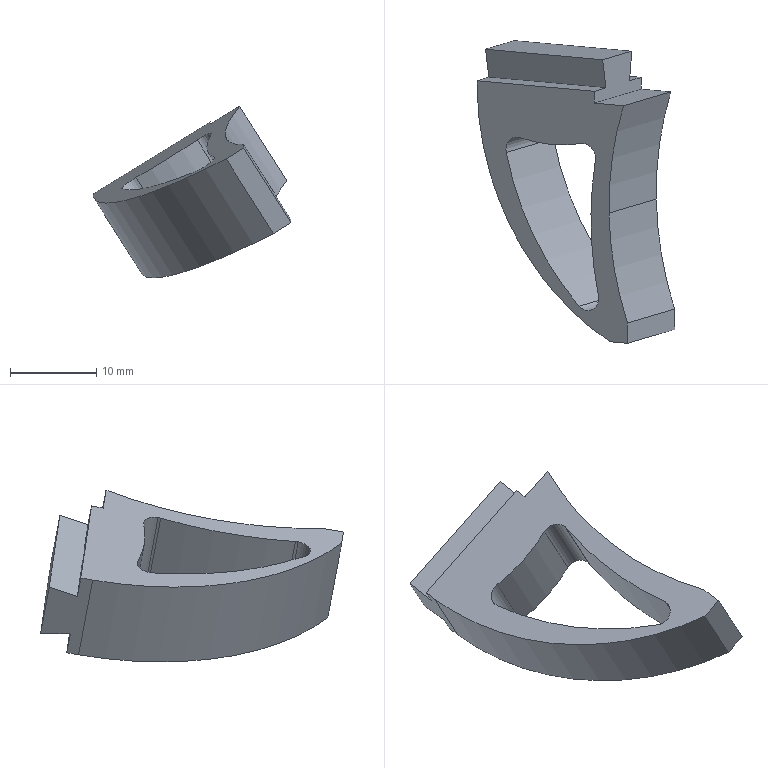Part | SolidWorks | features SplitBody 1 | 1 solid | 23 faces | box 22.985 x 35.159 x 19.952 mm | volume 2822 mm3 | plane 12 | cylinder 11 | commonest cylinder face diameters 3.2 x5 75.2 x2 40 x1 63.431 x1 67.2 x1 80 x1
STEP:
#1=CARTESIAN_POINT('',(526.695,281.026,-373.992));
#2=VERTEX_POINT('',#1);
#3=CARTESIAN_POINT('',(526.675,280.725,-374.062));
#4=VERTEX_POINT('',#3);
#5=CARTESIAN_POINT('',(525.336,281.15,-374.827));
#6=DIRECTION('',(0.5274,0.157,-0.835));
#7=DIRECTION('',(0.8494,-0.07732,0.522));
#8=AXIS2_PLACEMENT_3D('',#5,#6,#7);
#9=CIRCLE('',#8,1.6);
#10=EDGE_CURVE('',#2,#4,#9,.T.);
#11=ORIENTED_EDGE('',*,*,#10,.F.);
#12=CARTESIAN_POINT('',(532.181,282.659,-382.676));
#13=VERTEX_POINT('',#12);
#14=CARTESIAN_POINT('',(526.695,281.026,-373.992));
#15=DIRECTION('',(0.5274,0.157,-0.835));
#16=VECTOR('',#15,1000.);
#17=LINE('',#14,#16);
#18=EDGE_CURVE('',#2,#13,#17,.T.);
#19=ORIENTED_EDGE('',*,*,#18,.T.);
#20=CARTESIAN_POINT('',(532.161,282.358,-382.745));
#21=VERTEX_POINT('',#20);
#22=CARTESIAN_POINT('',(530.822,282.783,-383.511));
#23=DIRECTION('',(0.5274,0.157,-0.835));
#24=DIRECTION('',(0.8494,-0.07732,0.522));
#25=AXIS2_PLACEMENT_3D('',#22,#23,#24);
#26=CIRCLE('',#25,1.6);
#27=EDGE_CURVE('',#13,#21,#26,.T.);
#28=ORIENTED_EDGE('',*,*,#27,.T.);
#29=CARTESIAN_POINT('',(526.675,280.725,-374.062));
#30=DIRECTION('',(0.5274,0.157,-0.835));
#31=VECTOR('',#30,1000.);
#32=LINE('',#29,#31);
#33=EDGE_CURVE('',#4,#21,#32,.T.);
#34=ORIENTED_EDGE('',*,*,#33,.F.);
#35=EDGE_LOOP('',(#11,#19,#28,#34));
#36=FACE_OUTER_BOUND('',#35,.T.);
#37=CARTESIAN_POINT('',(525.336,281.15,-374.827));
#38=DIRECTION('',(0.5274,0.157,-0.835));
#39=DIRECTION('',(0.8494,-0.07732,0.522));
#40=AXIS2_PLACEMENT_3D('',#37,#38,#39);
#41=CYLINDRICAL_SURFACE('',#40,1.6);
#42=ADVANCED_FACE('',(#36),#41,.F.);
#43=CARTESIAN_POINT('',(524.781,263.843,-378.433));
#44=VERTEX_POINT('',#43);
#45=CARTESIAN_POINT('',(527.063,264.768,-376.818));
#46=VERTEX_POINT('',#45);
#47=CARTESIAN_POINT('',(525.703,264.892,-377.653));
#48=DIRECTION('',(-0.5274,-0.157,0.835));
#49=DIRECTION('',(0.8494,-0.07732,0.522));
#50=AXIS2_PLACEMENT_3D('',#47,#48,#49);
#51=CIRCLE('',#50,1.6);
#52=EDGE_CURVE('',#44,#46,#51,.T.);
#53=ORIENTED_EDGE('',*,*,#52,.T.);
#54=CARTESIAN_POINT('',(532.548,266.401,-385.501));
#55=VERTEX_POINT('',#54);
#56=CARTESIAN_POINT('',(527.063,264.768,-376.818));
#57=DIRECTION('',(0.5274,0.157,-0.835));
#58=VECTOR('',#57,1000.);
#59=LINE('',#56,#58);
#60=EDGE_CURVE('',#46,#55,#59,.T.);
#61=ORIENTED_EDGE('',*,*,#60,.T.);
#62=CARTESIAN_POINT('',(530.266,265.476,-387.117));
#63=VERTEX_POINT('',#62);
#64=CARTESIAN_POINT('',(531.189,266.525,-386.337));
#65=DIRECTION('',(-0.5274,-0.157,0.835));
#66=DIRECTION('',(0.8494,-0.07732,0.522));
#67=AXIS2_PLACEMENT_3D('',#64,#65,#66);
#68=CIRCLE('',#67,1.6);
#69=EDGE_CURVE('',#63,#55,#68,.T.);
#70=ORIENTED_EDGE('',*,*,#69,.F.);
#71=CARTESIAN_POINT('',(524.781,263.843,-378.433));
#72=DIRECTION('',(0.5274,0.157,-0.835));
#73=VECTOR('',#72,1000.);
#74=LINE('',#71,#73);
#75=EDGE_CURVE('',#44,#63,#74,.T.);
#76=ORIENTED_EDGE('',*,*,#75,.F.);
#77=EDGE_LOOP('',(#53,#61,#70,#76));
#78=FACE_OUTER_BOUND('',#77,.T.);
#79=CARTESIAN_POINT('',(525.703,264.892,-377.653));
#80=DIRECTION('',(0.5274,0.157,-0.835));
#81=DIRECTION('',(0.8494,-0.07732,0.522));
#82=AXIS2_PLACEMENT_3D('',#79,#80,#81);
#83=CYLINDRICAL_SURFACE('',#82,1.6);
#84=ADVANCED_FACE('',(#78),#83,.F.);
#85=CARTESIAN_POINT('',(533.75,276.287,-382.883));
#86=VERTEX_POINT('',#85);
#87=CARTESIAN_POINT('',(535.88,263.511,-383.94));
#88=VERTEX_POINT('',#87);
#89=CARTESIAN_POINT('',(565.688,273.38,-363.255));
#90=DIRECTION('',(-0.5274,-0.157,0.835));
#91=DIRECTION('',(0.8494,-0.07732,0.522));
#92=AXIS2_PLACEMENT_3D('',#89,#90,#91);
#93=CIRCLE('',#92,37.6);
#94=EDGE_CURVE('',#86,#88,#93,.T.);
#95=ORIENTED_EDGE('',*,*,#94,.F.);
#96=CARTESIAN_POINT('',(528.264,274.654,-374.199));
#97=VERTEX_POINT('',#96);
#98=CARTESIAN_POINT('',(533.75,276.287,-382.883));
#99=DIRECTION('',(-0.5274,-0.157,0.835));
#100=VECTOR('',#99,1000.);
#101=LINE('',#98,#100);
#102=EDGE_CURVE('',#86,#97,#101,.T.);
#103=ORIENTED_EDGE('',*,*,#102,.T.);
#104=CARTESIAN_POINT('',(530.395,261.878,-375.256));
#105=VERTEX_POINT('',#104);
#106=CARTESIAN_POINT('',(560.203,271.747,-354.571));
#107=DIRECTION('',(-0.5274,-0.157,0.835));
#108=DIRECTION('',(0.8494,-0.07732,0.522));
#109=AXIS2_PLACEMENT_3D('',#106,#107,#108);
#110=CIRCLE('',#109,37.6);
#111=EDGE_CURVE('',#97,#105,#110,.T.);
#112=ORIENTED_EDGE('',*,*,#111,.T.);
#113=CARTESIAN_POINT('',(535.88,263.511,-383.94));
#114=DIRECTION('',(-0.5274,-0.157,0.835));
#115=VECTOR('',#114,1000.);
#116=LINE('',#113,#115);
#117=EDGE_CURVE('',#88,#105,#116,.T.);
#118=ORIENTED_EDGE('',*,*,#117,.F.);
#119=EDGE_LOOP('',(#95,#103,#112,#118));
#120=FACE_OUTER_BOUND('',#119,.T.);
#121=CARTESIAN_POINT('',(565.688,273.38,-363.255));
#122=DIRECTION('',(-0.5274,-0.157,0.835));
#123=DIRECTION('',(-0.8494,0.07732,-0.522));
#124=AXIS2_PLACEMENT_3D('',#121,#122,#123);
#125=CYLINDRICAL_SURFACE('',#124,37.6);
#126=ADVANCED_FACE('',(#120),#125,.F.);
#127=CARTESIAN_POINT('',(512.961,288.629,-381.238));
#128=VERTEX_POINT('',#127);
#129=CARTESIAN_POINT('',(528.398,259.701,-376.927));
#130=VERTEX_POINT('',#129);
#131=CARTESIAN_POINT('',(539.892,286.573,-364.613));
#132=DIRECTION('',(-0.5274,-0.157,0.835));
#133=DIRECTION('',(0.8494,-0.07732,0.522));
#134=AXIS2_PLACEMENT_3D('',#131,#132,#133);
#135=CIRCLE('',#134,31.716);
#136=EDGE_CURVE('',#128,#130,#135,.T.);
#137=ORIENTED_EDGE('',*,*,#136,.F.);
#138=CARTESIAN_POINT('',(518.446,290.262,-389.922));
#139=VERTEX_POINT('',#138);
#140=CARTESIAN_POINT('',(518.446,290.262,-389.922));
#141=DIRECTION('',(-0.5274,-0.157,0.835));
#142=VECTOR('',#141,1000.);
#143=LINE('',#140,#142);
#144=EDGE_CURVE('',#139,#128,#143,.T.);
#145=ORIENTED_EDGE('',*,*,#144,.F.);
#146=CARTESIAN_POINT('',(533.883,261.334,-385.611));
#147=VERTEX_POINT('',#146);
#148=CARTESIAN_POINT('',(545.377,288.206,-373.297));
#149=DIRECTION('',(-0.5274,-0.157,0.835));
#150=DIRECTION('',(0.8494,-0.07732,0.522));
#151=AXIS2_PLACEMENT_3D('',#148,#149,#150);
#152=CIRCLE('',#151,31.716);
#153=EDGE_CURVE('',#139,#147,#152,.T.);
#154=ORIENTED_EDGE('',*,*,#153,.T.);
#155=CARTESIAN_POINT('',(533.883,261.334,-385.611));
#156=DIRECTION('',(-0.5274,-0.157,0.835));
#157=VECTOR('',#156,1000.);
#158=LINE('',#155,#157);
#159=EDGE_CURVE('',#147,#130,#158,.T.);
#160=ORIENTED_EDGE('',*,*,#159,.T.);
#161=EDGE_LOOP('',(#137,#145,#154,#160));
#162=FACE_OUTER_BOUND('',#161,.T.);
#163=CARTESIAN_POINT('',(545.377,288.206,-373.297));
#164=DIRECTION('',(-0.5274,-0.157,0.835));
#165=DIRECTION('',(-0.8494,0.07732,-0.522));
#166=AXIS2_PLACEMENT_3D('',#163,#164,#165);
#167=CYLINDRICAL_SURFACE('',#166,31.716);
#168=ADVANCED_FACE('',(#162),#167,.T.);
#169=CARTESIAN_POINT('',(517.051,291.23,-387.508));
#170=VERTEX_POINT('',#169);
#171=CARTESIAN_POINT('',(517.308,294.674,-387.416));
#172=VERTEX_POINT('',#171);
#173=CARTESIAN_POINT('',(517.051,291.23,-387.508));
#174=DIRECTION('',(0.07444,0.9969,0.02652));
#175=VECTOR('',#174,1000.);
#176=LINE('',#173,#175);
#177=EDGE_CURVE('',#170,#172,#176,.T.);
#178=ORIENTED_EDGE('',*,*,#177,.F.);
#179=CARTESIAN_POINT('',(518.422,291.638,-389.679));
#180=VERTEX_POINT('',#179);
#181=CARTESIAN_POINT('',(518.422,291.638,-389.679));
#182=DIRECTION('',(-0.5274,-0.157,0.835));
#183=VECTOR('',#182,1000.);
#184=LINE('',#181,#183);
#185=EDGE_CURVE('',#180,#170,#184,.T.);
#186=ORIENTED_EDGE('',*,*,#185,.F.);
#187=CARTESIAN_POINT('',(518.363,294.988,-389.086));
#188=DIRECTION('',(0.01741,-0.9846,-0.1742));
#189=VECTOR('',#188,1000.);
#190=LINE('',#187,#189);
#191=EDGE_CURVE('',#180,#139,#190,.T.);
#192=ORIENTED_EDGE('',*,*,#191,.T.);
#193=ORIENTED_EDGE('',*,*,#144,.T.);
#194=CARTESIAN_POINT('',(512.937,290.005,-380.995));
#195=VERTEX_POINT('',#194);
#196=CARTESIAN_POINT('',(512.877,293.355,-380.402));
#197=DIRECTION('',(0.01741,-0.9846,-0.1742));
#198=VECTOR('',#197,1000.);
#199=LINE('',#196,#198);
#200=EDGE_CURVE('',#195,#128,#199,.T.);
#201=ORIENTED_EDGE('',*,*,#200,.F.);
#202=CARTESIAN_POINT('',(514.308,290.413,-383.166));
#203=VERTEX_POINT('',#202);
#204=CARTESIAN_POINT('',(512.937,290.005,-380.995));
#205=DIRECTION('',(-0.5274,-0.157,0.835));
#206=VECTOR('',#205,1000.);
#207=LINE('',#204,#206);
#208=EDGE_CURVE('',#203,#195,#207,.T.);
#209=ORIENTED_EDGE('',*,*,#208,.F.);
#210=CARTESIAN_POINT('',(513.932,293.669,-382.072));
#211=VERTEX_POINT('',#210);
#212=CARTESIAN_POINT('',(514.308,290.413,-383.166));
#213=DIRECTION('',(0.1087,-0.9423,-0.3165));
#214=VECTOR('',#213,1000.);
#215=LINE('',#212,#214);
#216=EDGE_CURVE('',#211,#203,#215,.T.);
#217=ORIENTED_EDGE('',*,*,#216,.F.);
#218=CARTESIAN_POINT('',(518.363,294.988,-389.086));
#219=DIRECTION('',(-0.5274,-0.157,0.835));
#220=VECTOR('',#219,1000.);
#221=LINE('',#218,#220);
#222=EDGE_CURVE('',#172,#211,#221,.T.);
#223=ORIENTED_EDGE('',*,*,#222,.F.);
#224=EDGE_LOOP('',(#178,#186,#192,#193,#201,#209,#217,#223));
#225=FACE_OUTER_BOUND('',#224,.T.);
#226=CARTESIAN_POINT('',(518.363,294.988,-389.086));
#227=DIRECTION('',(-0.8494,0.07732,-0.522));
#228=DIRECTION('',(0.5274,0.157,-0.835));
#229=AXIS2_PLACEMENT_3D('',#226,#227,#228);
#230=PLANE('',#229);
#231=ADVANCED_FACE('',(#225),#230,.T.);
#232=CARTESIAN_POINT('',(530.899,293.437,-379.064));
#233=VERTEX_POINT('',#232);
#234=CARTESIAN_POINT('',(527.523,292.432,-373.72));
#235=VERTEX_POINT('',#234);
#236=CARTESIAN_POINT('',(531.953,293.751,-380.734));
#237=DIRECTION('',(-0.5274,-0.157,0.835));
#238=VECTOR('',#237,1000.);
#239=LINE('',#236,#238);
#240=EDGE_CURVE('',#233,#235,#239,.T.);
#241=ORIENTED_EDGE('',*,*,#240,.F.);
#242=CARTESIAN_POINT('',(534.296,293.128,-376.976));
#243=DIRECTION('',(-0.8494,0.07732,-0.522));
#244=VECTOR('',#243,1000.);
#245=LINE('',#242,#244);
#246=EDGE_CURVE('',#233,#172,#245,.T.);
#247=ORIENTED_EDGE('',*,*,#246,.T.);
#248=ORIENTED_EDGE('',*,*,#222,.T.);
#249=CARTESIAN_POINT('',(530.921,292.123,-371.632));
#250=DIRECTION('',(-0.8494,0.07732,-0.522));
#251=VECTOR('',#250,1000.);
#252=LINE('',#249,#251);
#253=EDGE_CURVE('',#235,#211,#252,.T.);
#254=ORIENTED_EDGE('',*,*,#253,.F.);
#255=EDGE_LOOP('',(#241,#247,#248,#254));
#256=FACE_OUTER_BOUND('',#255,.T.);
#257=CARTESIAN_POINT('',(518.363,294.988,-389.086));
#258=DIRECTION('',(0.01741,-0.9846,-0.1742));
#259=DIRECTION('',(-0.8494,0.07732,-0.522));
#260=AXIS2_PLACEMENT_3D('',#257,#258,#259);
#261=PLANE('',#260);
#262=ADVANCED_FACE('',(#256),#261,.F.);
#263=CARTESIAN_POINT('',(532.013,290.401,-381.326));
#264=VERTEX_POINT('',#263);
#265=CARTESIAN_POINT('',(530.641,289.992,-379.155));
#266=VERTEX_POINT('',#265);
#267=CARTESIAN_POINT('',(532.013,290.401,-381.326));
#268=DIRECTION('',(-0.5274,-0.157,0.835));
#269=VECTOR('',#268,1000.);
#270=LINE('',#267,#269);
#271=EDGE_CURVE('',#264,#266,#270,.T.);
#272=ORIENTED_EDGE('',*,*,#271,.T.);
#273=CARTESIAN_POINT('',(530.924,293.783,-379.054));
#274=DIRECTION('',(0.07444,0.9969,0.02652));
#275=VECTOR('',#274,1000.);
#276=LINE('',#273,#275);
#277=EDGE_CURVE('',#266,#233,#276,.T.);
#278=ORIENTED_EDGE('',*,*,#277,.T.);
#279=ORIENTED_EDGE('',*,*,#240,.T.);
#280=CARTESIAN_POINT('',(527.899,289.176,-374.814));
#281=VERTEX_POINT('',#280);
#282=CARTESIAN_POINT('',(527.682,291.057,-374.182));
#283=DIRECTION('',(0.1087,-0.9423,-0.3165));
#284=VECTOR('',#283,1000.);
#285=LINE('',#282,#284);
#286=EDGE_CURVE('',#235,#281,#285,.T.);
#287=ORIENTED_EDGE('',*,*,#286,.T.);
#288=CARTESIAN_POINT('',(526.527,288.768,-372.643));
#289=VERTEX_POINT('',#288);
#290=CARTESIAN_POINT('',(532.013,290.401,-381.326));
#291=DIRECTION('',(-0.5274,-0.157,0.835));
#292=VECTOR('',#291,1000.);
#293=LINE('',#290,#292);
#294=EDGE_CURVE('',#281,#289,#293,.T.);
#295=ORIENTED_EDGE('',*,*,#294,.T.);
#296=CARTESIAN_POINT('',(526.552,287.392,-372.886));
#297=VERTEX_POINT('',#296);
#298=CARTESIAN_POINT('',(526.468,292.118,-372.05));
#299=DIRECTION('',(0.01741,-0.9846,-0.1742));
#300=VECTOR('',#299,1000.);
#301=LINE('',#298,#300);
#302=EDGE_CURVE('',#289,#297,#301,.T.);
#303=ORIENTED_EDGE('',*,*,#302,.T.);
#304=CARTESIAN_POINT('',(532.037,289.025,-381.57));
#305=VERTEX_POINT('',#304);
#306=CARTESIAN_POINT('',(532.037,289.025,-381.57));
#307=DIRECTION('',(-0.5274,-0.157,0.835));
#308=VECTOR('',#307,1000.);
#309=LINE('',#306,#308);
#310=EDGE_CURVE('',#305,#297,#309,.T.);
#311=ORIENTED_EDGE('',*,*,#310,.F.);
#312=CARTESIAN_POINT('',(531.953,293.751,-380.734));
#313=DIRECTION('',(0.01741,-0.9846,-0.1742));
#314=VECTOR('',#313,1000.);
#315=LINE('',#312,#314);
#316=EDGE_CURVE('',#264,#305,#315,.T.);
#317=ORIENTED_EDGE('',*,*,#316,.F.);
#318=EDGE_LOOP('',(#272,#278,#279,#287,#295,#303,#311,#317));
#319=FACE_OUTER_BOUND('',#318,.T.);
#320=CARTESIAN_POINT('',(531.953,293.751,-380.734));
#321=DIRECTION('',(-0.8494,0.07732,-0.522));
#322=DIRECTION('',(0.5274,0.157,-0.835));
#323=AXIS2_PLACEMENT_3D('',#320,#321,#322);
#324=PLANE('',#323);
#325=ADVANCED_FACE('',(#319),#324,.F.);
#326=CARTESIAN_POINT('',(529.949,287.083,-370.798));
#327=VERTEX_POINT('',#326);
#328=CARTESIAN_POINT('',(512.961,288.629,-381.238));
#329=DIRECTION('',(0.8494,-0.07732,0.522));
#330=VECTOR('',#329,1000.);
#331=LINE('',#328,#330);
#332=EDGE_CURVE('',#297,#327,#331,.T.);
#333=ORIENTED_EDGE('',*,*,#332,.T.);
#334=CARTESIAN_POINT('',(535.435,288.716,-379.481));
#335=VERTEX_POINT('',#334);
#336=CARTESIAN_POINT('',(535.435,288.716,-379.481));
#337=DIRECTION('',(-0.5274,-0.157,0.835));
#338=VECTOR('',#337,1000.);
#339=LINE('',#336,#338);
#340=EDGE_CURVE('',#335,#327,#339,.T.);
#341=ORIENTED_EDGE('',*,*,#340,.F.);
#342=CARTESIAN_POINT('',(518.446,290.262,-389.922));
#343=DIRECTION('',(0.8494,-0.07732,0.522));
#344=VECTOR('',#343,1000.);
#345=LINE('',#342,#344);
#346=EDGE_CURVE('',#305,#335,#345,.T.);
#347=ORIENTED_EDGE('',*,*,#346,.F.);
#348=ORIENTED_EDGE('',*,*,#310,.T.);
#349=EDGE_LOOP('',(#333,#341,#347,#348));
#350=FACE_OUTER_BOUND('',#349,.T.);
#351=CARTESIAN_POINT('',(518.446,290.262,-389.922));
#352=DIRECTION('',(0.01741,-0.9846,-0.1742));
#353=DIRECTION('',(-0.8494,0.07732,-0.522));
#354=AXIS2_PLACEMENT_3D('',#351,#352,#353);
#355=PLANE('',#354);
#356=ADVANCED_FACE('',(#350),#355,.F.);
#357=ORIENTED_EDGE('',*,*,#102,.F.);
#358=CARTESIAN_POINT('',(565.688,273.38,-363.255));
#359=DIRECTION('',(-0.5274,-0.157,0.835));
#360=DIRECTION('',(0.8494,-0.07732,0.522));
#361=AXIS2_PLACEMENT_3D('',#358,#359,#360);
#362=CIRCLE('',#361,37.6);
#363=EDGE_CURVE('',#335,#86,#362,.T.);
#364=ORIENTED_EDGE('',*,*,#363,.F.);
#365=ORIENTED_EDGE('',*,*,#340,.T.);
#366=CARTESIAN_POINT('',(560.203,271.747,-354.571));
#367=DIRECTION('',(-0.5274,-0.157,0.835));
#368=DIRECTION('',(0.8494,-0.07732,0.522));
#369=AXIS2_PLACEMENT_3D('',#366,#367,#368);
#370=CIRCLE('',#369,37.6);
#371=EDGE_CURVE('',#327,#97,#370,.T.);
#372=ORIENTED_EDGE('',*,*,#371,.T.);
#373=EDGE_LOOP('',(#357,#364,#365,#372));
#374=FACE_OUTER_BOUND('',#373,.T.);
#375=CARTESIAN_POINT('',(565.688,273.38,-363.255));
#376=DIRECTION('',(-0.5274,-0.157,0.835));
#377=DIRECTION('',(-0.8494,0.07732,-0.522));
#378=AXIS2_PLACEMENT_3D('',#375,#376,#377);
#379=CYLINDRICAL_SURFACE('',#378,37.6);
#380=ADVANCED_FACE('',(#374),#379,.F.);
#381=CARTESIAN_POINT('',(530.437,259.515,-375.674));
#382=VERTEX_POINT('',#381);
#383=CARTESIAN_POINT('',(529.866,291.809,-369.962));
#384=DIRECTION('',(0.01741,-0.9846,-0.1742));
#385=VECTOR('',#384,1000.);
#386=LINE('',#383,#385);
#387=EDGE_CURVE('',#105,#382,#386,.T.);
#388=ORIENTED_EDGE('',*,*,#387,.T.);
#389=CARTESIAN_POINT('',(535.922,261.148,-384.358));
#390=VERTEX_POINT('',#389);
#391=CARTESIAN_POINT('',(535.922,261.148,-384.358));
#392=DIRECTION('',(-0.5274,-0.157,0.835));
#393=VECTOR('',#392,1000.);
#394=LINE('',#391,#393);
#395=EDGE_CURVE('',#390,#382,#394,.T.);
#396=ORIENTED_EDGE('',*,*,#395,.F.);
#397=CARTESIAN_POINT('',(535.351,293.442,-378.645));
#398=DIRECTION('',(0.01741,-0.9846,-0.1742));
#399=VECTOR('',#398,1000.);
#400=LINE('',#397,#399);
#401=EDGE_CURVE('',#88,#390,#400,.T.);
#402=ORIENTED_EDGE('',*,*,#401,.F.);
#403=ORIENTED_EDGE('',*,*,#117,.T.);
#404=EDGE_LOOP('',(#388,#396,#402,#403));
#405=FACE_OUTER_BOUND('',#404,.T.);
#406=CARTESIAN_POINT('',(535.351,293.442,-378.645));
#407=DIRECTION('',(-0.8494,0.07732,-0.522));
#408=DIRECTION('',(0.5274,0.157,-0.835));
#409=AXIS2_PLACEMENT_3D('',#406,#407,#408);
#410=PLANE('',#409);
#411=ADVANCED_FACE('',(#405),#410,.F.);
#412=CARTESIAN_POINT('',(513.448,261.061,-386.115));
#413=DIRECTION('',(-0.8494,0.07732,-0.522));
#414=VECTOR('',#413,1000.);
#415=LINE('',#412,#414);
#416=EDGE_CURVE('',#382,#130,#415,.T.);
#417=ORIENTED_EDGE('',*,*,#416,.T.);
#418=ORIENTED_EDGE('',*,*,#159,.F.);
#419=CARTESIAN_POINT('',(518.934,262.694,-394.798));
#420=DIRECTION('',(-0.8494,0.07732,-0.522));
#421=VECTOR('',#420,1000.);
#422=LINE('',#419,#421);
#423=EDGE_CURVE('',#390,#147,#422,.T.);
#424=ORIENTED_EDGE('',*,*,#423,.F.);
#425=ORIENTED_EDGE('',*,*,#395,.T.);
#426=EDGE_LOOP('',(#417,#418,#424,#425));
#427=FACE_OUTER_BOUND('',#426,.T.);
#428=CARTESIAN_POINT('',(518.934,262.694,-394.798));
#429=DIRECTION('',(-0.01741,0.9846,0.1742));
#430=DIRECTION('',(0.8494,-0.07732,0.522));
#431=AXIS2_PLACEMENT_3D('',#428,#429,#430);
#432=PLANE('',#431);
#433=ADVANCED_FACE('',(#427),#432,.F.);
#434=CARTESIAN_POINT('',(521.816,283.318,-389.1));
#435=VERTEX_POINT('',#434);
#436=CARTESIAN_POINT('',(549.64,287.505,-370.736));
#437=DIRECTION('',(-0.5274,-0.157,0.835));
#438=DIRECTION('',(0.8494,-0.07732,0.522));
#439=AXIS2_PLACEMENT_3D('',#436,#437,#438);
#440=CIRCLE('',#439,33.6);
#441=EDGE_CURVE('',#435,#63,#440,.T.);
#442=ORIENTED_EDGE('',*,*,#441,.T.);
#443=ORIENTED_EDGE('',*,*,#69,.T.);
#444=CARTESIAN_POINT('',(532.514,266.725,-385.462));
#445=VERTEX_POINT('',#444);
#446=CARTESIAN_POINT('',(531.189,266.525,-386.337));
#447=DIRECTION('',(-0.5274,-0.157,0.835));
#448=DIRECTION('',(0.8494,-0.07732,0.522));
#449=AXIS2_PLACEMENT_3D('',#446,#447,#448);
#450=CIRCLE('',#449,1.6);
#451=EDGE_CURVE('',#55,#445,#450,.T.);
#452=ORIENTED_EDGE('',*,*,#451,.T.);
#453=CARTESIAN_POINT('',(565.634,271.73,-363.599));
#454=DIRECTION('',(0.5274,0.157,-0.835));
#455=DIRECTION('',(0.8494,-0.07732,0.522));
#456=AXIS2_PLACEMENT_3D('',#453,#454,#455);
#457=CIRCLE('',#456,40.);
#458=EDGE_CURVE('',#445,#21,#457,.T.);
#459=ORIENTED_EDGE('',*,*,#458,.T.);
#460=ORIENTED_EDGE('',*,*,#27,.F.);
#461=CARTESIAN_POINT('',(530.515,284.35,-383.41));
#462=VERTEX_POINT('',#461);
#463=CARTESIAN_POINT('',(530.822,282.783,-383.511));
#464=DIRECTION('',(0.5274,0.157,-0.835));
#465=DIRECTION('',(0.8494,-0.07732,0.522));
#466=AXIS2_PLACEMENT_3D('',#463,#464,#465);
#467=CIRCLE('',#466,1.6);
#468=EDGE_CURVE('',#462,#13,#467,.T.);
#469=ORIENTED_EDGE('',*,*,#468,.F.);
#470=CARTESIAN_POINT('',(523.403,285.031,-387.775));
#471=VERTEX_POINT('',#470);
#472=CARTESIAN_POINT('',(526.685,303.939,-382.146));
#473=DIRECTION('',(-0.5274,-0.157,0.835));
#474=DIRECTION('',(0.8494,-0.07732,0.522));
#475=AXIS2_PLACEMENT_3D('',#472,#473,#474);
#476=CIRCLE('',#475,20.);
#477=EDGE_CURVE('',#471,#462,#476,.T.);
#478=ORIENTED_EDGE('',*,*,#477,.F.);
#479=CARTESIAN_POINT('',(523.14,283.518,-388.225));
#480=DIRECTION('',(-0.5274,-0.157,0.835));
#481=DIRECTION('',(0.8494,-0.07732,0.522));
#482=AXIS2_PLACEMENT_3D('',#479,#480,#481);
#483=CIRCLE('',#482,1.6);
#484=EDGE_CURVE('',#471,#435,#483,.T.);
#485=ORIENTED_EDGE('',*,*,#484,.T.);
#486=EDGE_LOOP('',(#442,#443,#452,#459,#460,#469,#478,#485));
#487=FACE_BOUND('',#486,.T.);
#488=CARTESIAN_POINT('',(518.422,291.638,-389.679));
#489=DIRECTION('',(-0.8494,0.07732,-0.522));
#490=VECTOR('',#489,1000.);
#491=LINE('',#488,#490);
#492=EDGE_CURVE('',#264,#180,#491,.T.);
#493=ORIENTED_EDGE('',*,*,#492,.F.);
#494=ORIENTED_EDGE('',*,*,#316,.T.);
#495=ORIENTED_EDGE('',*,*,#346,.T.);
#496=ORIENTED_EDGE('',*,*,#363,.T.);
#497=ORIENTED_EDGE('',*,*,#94,.T.);
#498=ORIENTED_EDGE('',*,*,#401,.T.);
#499=ORIENTED_EDGE('',*,*,#423,.T.);
#500=ORIENTED_EDGE('',*,*,#153,.F.);
#501=ORIENTED_EDGE('',*,*,#191,.F.);
#502=EDGE_LOOP('',(#493,#494,#495,#496,#497,#498,#499,#500,#501));
#503=FACE_OUTER_BOUND('',#502,.T.);
#504=CARTESIAN_POINT('',(518.363,294.988,-389.086));
#505=DIRECTION('',(0.5274,0.157,-0.835));
#506=DIRECTION('',(0.8494,-0.07732,0.522));
#507=AXIS2_PLACEMENT_3D('',#504,#505,#506);
#508=PLANE('',#507);
#509=ADVANCED_FACE('',(#487,#503),#508,.T.);
#510=ORIENTED_EDGE('',*,*,#52,.F.);
#511=CARTESIAN_POINT('',(516.33,281.685,-380.416));
#512=VERTEX_POINT('',#511);
#513=CARTESIAN_POINT('',(544.155,285.872,-362.052));
#514=DIRECTION('',(-0.5274,-0.157,0.835));
#515=DIRECTION('',(0.8494,-0.07732,0.522));
#516=AXIS2_PLACEMENT_3D('',#513,#514,#515);
#517=CIRCLE('',#516,33.6);
#518=EDGE_CURVE('',#512,#44,#517,.T.);
#519=ORIENTED_EDGE('',*,*,#518,.F.);
#520=CARTESIAN_POINT('',(517.918,283.398,-379.091));
#521=VERTEX_POINT('',#520);
#522=CARTESIAN_POINT('',(517.655,281.885,-379.541));
#523=DIRECTION('',(-0.5274,-0.157,0.835));
#524=DIRECTION('',(0.8494,-0.07732,0.522));
#525=AXIS2_PLACEMENT_3D('',#522,#523,#524);
#526=CIRCLE('',#525,1.6);
#527=EDGE_CURVE('',#521,#512,#526,.T.);
#528=ORIENTED_EDGE('',*,*,#527,.F.);
#529=CARTESIAN_POINT('',(525.03,282.717,-374.726));
#530=VERTEX_POINT('',#529);
#531=CARTESIAN_POINT('',(521.2,302.306,-373.462));
#532=DIRECTION('',(-0.5274,-0.157,0.835));
#533=DIRECTION('',(0.8494,-0.07732,0.522));
#534=AXIS2_PLACEMENT_3D('',#531,#532,#533);
#535=CIRCLE('',#534,20.);
#536=EDGE_CURVE('',#521,#530,#535,.T.);
#537=ORIENTED_EDGE('',*,*,#536,.T.);
#538=CARTESIAN_POINT('',(525.336,281.15,-374.827));
#539=DIRECTION('',(0.5274,0.157,-0.835));
#540=DIRECTION('',(0.8494,-0.07732,0.522));
#541=AXIS2_PLACEMENT_3D('',#538,#539,#540);
#542=CIRCLE('',#541,1.6);
#543=EDGE_CURVE('',#530,#2,#542,.T.);
#544=ORIENTED_EDGE('',*,*,#543,.T.);
#545=ORIENTED_EDGE('',*,*,#10,.T.);
#546=CARTESIAN_POINT('',(527.028,265.092,-376.779));
#547=VERTEX_POINT('',#546);
#548=CARTESIAN_POINT('',(560.149,270.097,-354.916));
#549=DIRECTION('',(0.5274,0.157,-0.835));
#550=DIRECTION('',(0.8494,-0.07732,0.522));
#551=AXIS2_PLACEMENT_3D('',#548,#549,#550);
#552=CIRCLE('',#551,40.);
#553=EDGE_CURVE('',#547,#4,#552,.T.);
#554=ORIENTED_EDGE('',*,*,#553,.F.);
#555=CARTESIAN_POINT('',(525.703,264.892,-377.653));
#556=DIRECTION('',(-0.5274,-0.157,0.835));
#557=DIRECTION('',(0.8494,-0.07732,0.522));
#558=AXIS2_PLACEMENT_3D('',#555,#556,#557);
#559=CIRCLE('',#558,1.6);
#560=EDGE_CURVE('',#46,#547,#559,.T.);
#561=ORIENTED_EDGE('',*,*,#560,.F.);
#562=EDGE_LOOP('',(#510,#519,#528,#537,#544,#545,#554,#561));
#563=FACE_BOUND('',#562,.T.);
#564=ORIENTED_EDGE('',*,*,#302,.F.);
#565=CARTESIAN_POINT('',(512.937,290.005,-380.995));
#566=DIRECTION('',(-0.8494,0.07732,-0.522));
#567=VECTOR('',#566,1000.);
#568=LINE('',#565,#567);
#569=EDGE_CURVE('',#289,#195,#568,.T.);
#570=ORIENTED_EDGE('',*,*,#569,.T.);
#571=ORIENTED_EDGE('',*,*,#200,.T.);
#572=ORIENTED_EDGE('',*,*,#136,.T.);
#573=ORIENTED_EDGE('',*,*,#416,.F.);
#574=ORIENTED_EDGE('',*,*,#387,.F.);
#575=ORIENTED_EDGE('',*,*,#111,.F.);
#576=ORIENTED_EDGE('',*,*,#371,.F.);
#577=ORIENTED_EDGE('',*,*,#332,.F.);
#578=EDGE_LOOP('',(#564,#570,#571,#572,#573,#574,#575,#576,#577));
#579=FACE_OUTER_BOUND('',#578,.T.);
#580=CARTESIAN_POINT('',(512.877,293.355,-380.402));
#581=DIRECTION('',(0.5274,0.157,-0.835));
#582=DIRECTION('',(0.8494,-0.07732,0.522));
#583=AXIS2_PLACEMENT_3D('',#580,#581,#582);
#584=PLANE('',#583);
#585=ADVANCED_FACE('',(#563,#579),#584,.F.);
#586=ORIENTED_EDGE('',*,*,#253,.T.);
#587=ORIENTED_EDGE('',*,*,#216,.T.);
#588=CARTESIAN_POINT('',(531.296,288.867,-372.725));
#589=DIRECTION('',(-0.8494,0.07732,-0.522));
#590=VECTOR('',#589,1000.);
#591=LINE('',#588,#590);
#592=EDGE_CURVE('',#281,#203,#591,.T.);
#593=ORIENTED_EDGE('',*,*,#592,.F.);
#594=ORIENTED_EDGE('',*,*,#286,.F.);
#595=EDGE_LOOP('',(#586,#587,#593,#594));
#596=FACE_OUTER_BOUND('',#595,.T.);
#597=CARTESIAN_POINT('',(531.296,288.867,-372.725));
#598=DIRECTION('',(0.5164,0.3256,-0.792));
#599=DIRECTION('',(0.1087,-0.9423,-0.3165));
#600=AXIS2_PLACEMENT_3D('',#597,#598,#599);
#601=PLANE('',#600);
#602=ADVANCED_FACE('',(#596),#601,.F.);
#603=ORIENTED_EDGE('',*,*,#592,.T.);
#604=ORIENTED_EDGE('',*,*,#208,.T.);
#605=ORIENTED_EDGE('',*,*,#569,.F.);
#606=ORIENTED_EDGE('',*,*,#294,.F.);
#607=EDGE_LOOP('',(#603,#604,#605,#606));
#608=FACE_OUTER_BOUND('',#607,.T.);
#609=CARTESIAN_POINT('',(529.925,288.458,-370.555));
#610=DIRECTION('',(0.01741,-0.9846,-0.1742));
#611=DIRECTION('',(-0.5274,-0.157,0.835));
#612=AXIS2_PLACEMENT_3D('',#609,#610,#611);
#613=PLANE('',#612);
#614=ADVANCED_FACE('',(#608),#613,.F.);
#615=CARTESIAN_POINT('',(534.039,289.683,-377.067));
#616=DIRECTION('',(-0.8494,0.07732,-0.522));
#617=VECTOR('',#616,1000.);
#618=LINE('',#615,#617);
#619=EDGE_CURVE('',#266,#170,#618,.T.);
#620=ORIENTED_EDGE('',*,*,#619,.T.);
#621=ORIENTED_EDGE('',*,*,#177,.T.);
#622=ORIENTED_EDGE('',*,*,#246,.F.);
#623=ORIENTED_EDGE('',*,*,#277,.F.);
#624=EDGE_LOOP('',(#620,#621,#622,#623));
#625=FACE_OUTER_BOUND('',#624,.T.);
#626=CARTESIAN_POINT('',(534.039,289.683,-377.067));
#627=DIRECTION('',(-0.5224,0.01633,0.8525));
#628=DIRECTION('',(0.07444,0.9969,0.02652));
#629=AXIS2_PLACEMENT_3D('',#626,#627,#628);
#630=PLANE('',#629);
#631=ADVANCED_FACE('',(#625),#630,.F.);
#632=ORIENTED_EDGE('',*,*,#492,.T.);
#633=ORIENTED_EDGE('',*,*,#185,.T.);
#634=ORIENTED_EDGE('',*,*,#619,.F.);
#635=ORIENTED_EDGE('',*,*,#271,.F.);
#636=EDGE_LOOP('',(#632,#633,#634,#635));
#637=FACE_OUTER_BOUND('',#636,.T.);
#638=CARTESIAN_POINT('',(535.41,290.091,-379.238));
#639=DIRECTION('',(0.01741,-0.9846,-0.1742));
#640=DIRECTION('',(-0.5274,-0.157,0.835));
#641=AXIS2_PLACEMENT_3D('',#638,#639,#640);
#642=PLANE('',#641);
#643=ADVANCED_FACE('',(#637),#642,.F.);
#644=ORIENTED_EDGE('',*,*,#60,.F.);
#645=ORIENTED_EDGE('',*,*,#560,.T.);
#646=CARTESIAN_POINT('',(527.028,265.092,-376.779));
#647=DIRECTION('',(0.5274,0.157,-0.835));
#648=VECTOR('',#647,1000.);
#649=LINE('',#646,#648);
#650=EDGE_CURVE('',#547,#445,#649,.T.);
#651=ORIENTED_EDGE('',*,*,#650,.T.);
#652=ORIENTED_EDGE('',*,*,#451,.F.);
#653=EDGE_LOOP('',(#644,#645,#651,#652));
#654=FACE_OUTER_BOUND('',#653,.T.);
#655=CARTESIAN_POINT('',(525.703,264.892,-377.653));
#656=DIRECTION('',(0.5274,0.157,-0.835));
#657=DIRECTION('',(0.8494,-0.07732,0.522));
#658=AXIS2_PLACEMENT_3D('',#655,#656,#657);
#659=CYLINDRICAL_SURFACE('',#658,1.6);
#660=ADVANCED_FACE('',(#654),#659,.F.);
#661=ORIENTED_EDGE('',*,*,#458,.F.);
#662=ORIENTED_EDGE('',*,*,#650,.F.);
#663=ORIENTED_EDGE('',*,*,#553,.T.);
#664=ORIENTED_EDGE('',*,*,#33,.T.);
#665=EDGE_LOOP('',(#661,#662,#663,#664));
#666=FACE_OUTER_BOUND('',#665,.T.);
#667=CARTESIAN_POINT('',(560.149,270.097,-354.916));
#668=DIRECTION('',(0.5274,0.157,-0.835));
#669=DIRECTION('',(0.8494,-0.07732,0.522));
#670=AXIS2_PLACEMENT_3D('',#667,#668,#669);
#671=CYLINDRICAL_SURFACE('',#670,40.);
#672=ADVANCED_FACE('',(#666),#671,.T.);
#673=ORIENTED_EDGE('',*,*,#18,.F.);
#674=ORIENTED_EDGE('',*,*,#543,.F.);
#675=CARTESIAN_POINT('',(525.03,282.717,-374.726));
#676=DIRECTION('',(0.5274,0.157,-0.835));
#677=VECTOR('',#676,1000.);
#678=LINE('',#675,#677);
#679=EDGE_CURVE('',#530,#462,#678,.T.);
#680=ORIENTED_EDGE('',*,*,#679,.T.);
#681=ORIENTED_EDGE('',*,*,#468,.T.);
#682=EDGE_LOOP('',(#673,#674,#680,#681));
#683=FACE_OUTER_BOUND('',#682,.T.);
#684=CARTESIAN_POINT('',(525.336,281.15,-374.827));
#685=DIRECTION('',(0.5274,0.157,-0.835));
#686=DIRECTION('',(0.8494,-0.07732,0.522));
#687=AXIS2_PLACEMENT_3D('',#684,#685,#686);
#688=CYLINDRICAL_SURFACE('',#687,1.6);
#689=ADVANCED_FACE('',(#683),#688,.F.);
#690=ORIENTED_EDGE('',*,*,#477,.T.);
#691=ORIENTED_EDGE('',*,*,#679,.F.);
#692=ORIENTED_EDGE('',*,*,#536,.F.);
#693=CARTESIAN_POINT('',(517.918,283.398,-379.091));
#694=DIRECTION('',(0.5274,0.157,-0.835));
#695=VECTOR('',#694,1000.);
#696=LINE('',#693,#695);
#697=EDGE_CURVE('',#521,#471,#696,.T.);
#698=ORIENTED_EDGE('',*,*,#697,.T.);
#699=EDGE_LOOP('',(#690,#691,#692,#698));
#700=FACE_OUTER_BOUND('',#699,.T.);
#701=CARTESIAN_POINT('',(521.2,302.306,-373.462));
#702=DIRECTION('',(0.5274,0.157,-0.835));
#703=DIRECTION('',(0.8494,-0.07732,0.522));
#704=AXIS2_PLACEMENT_3D('',#701,#702,#703);
#705=CYLINDRICAL_SURFACE('',#704,20.);
#706=ADVANCED_FACE('',(#700),#705,.T.);
#707=ORIENTED_EDGE('',*,*,#484,.F.);
#708=ORIENTED_EDGE('',*,*,#697,.F.);
#709=ORIENTED_EDGE('',*,*,#527,.T.);
#710=CARTESIAN_POINT('',(516.33,281.685,-380.416));
#711=DIRECTION('',(0.5274,0.157,-0.835));
#712=VECTOR('',#711,1000.);
#713=LINE('',#710,#712);
#714=EDGE_CURVE('',#512,#435,#713,.T.);
#715=ORIENTED_EDGE('',*,*,#714,.T.);
#716=EDGE_LOOP('',(#707,#708,#709,#715));
#717=FACE_OUTER_BOUND('',#716,.T.);
#718=CARTESIAN_POINT('',(517.655,281.885,-379.541));
#719=DIRECTION('',(0.5274,0.157,-0.835));
#720=DIRECTION('',(0.8494,-0.07732,0.522));
#721=AXIS2_PLACEMENT_3D('',#718,#719,#720);
#722=CYLINDRICAL_SURFACE('',#721,1.6);
#723=ADVANCED_FACE('',(#717),#722,.F.);
#724=ORIENTED_EDGE('',*,*,#441,.F.);
#725=ORIENTED_EDGE('',*,*,#714,.F.);
#726=ORIENTED_EDGE('',*,*,#518,.T.);
#727=ORIENTED_EDGE('',*,*,#75,.T.);
#728=EDGE_LOOP('',(#724,#725,#726,#727));
#729=FACE_OUTER_BOUND('',#728,.T.);
#730=CARTESIAN_POINT('',(544.155,285.872,-362.052));
#731=DIRECTION('',(0.5274,0.157,-0.835));
#732=DIRECTION('',(0.8494,-0.07732,0.522));
#733=AXIS2_PLACEMENT_3D('',#730,#731,#732);
#734=CYLINDRICAL_SURFACE('',#733,33.6);
#735=ADVANCED_FACE('',(#729),#734,.F.);
#736=CLOSED_SHELL('',(#42,#84,#126,#168,#231,#262,#325,#356,#380,#411,#433,#509,#585,#602,#614,#631,#643,#660,#672,#689,#706,#723,#735));
#737=MANIFOLD_SOLID_BREP('',#736);
#738=CARTESIAN_POINT('',(0.,0.,0.));
#739=DIRECTION('',(0.,0.,1.));
#740=DIRECTION('',(1.,0.,0.));
#741=AXIS2_PLACEMENT_3D('',#738,#739,#740);
#742=(LENGTH_UNIT()NAMED_UNIT(*)SI_UNIT(.MILLI.,.METRE.));
#743=UNCERTAINTY_MEASURE_WITH_UNIT(LENGTH_MEASURE(0.00001),#742,'','');
#744=(NAMED_UNIT(*)PLANE_ANGLE_UNIT()SI_UNIT($,.RADIAN.));
#745=(NAMED_UNIT(*)SI_UNIT($,.STERADIAN.)SOLID_ANGLE_UNIT());
#746=(GEOMETRIC_REPRESENTATION_CONTEXT(3)GLOBAL_UNCERTAINTY_ASSIGNED_CONTEXT((#743))GLOBAL_UNIT_ASSIGNED_CONTEXT((#742,#744,#745))REPRESENTATION_CONTEXT('',''));
#747=ADVANCED_BREP_SHAPE_REPRESENTATION('',(#737,#741),#746);